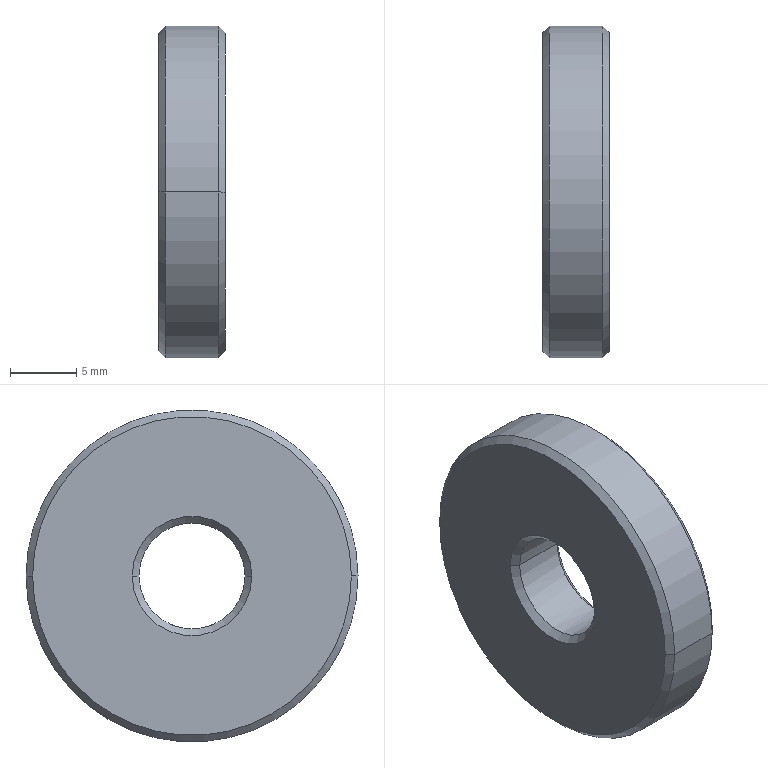Part | SolidWorks | features BaseBody 1 | 1 solid | 14 faces | box 5 x 25 x 25 mm | volume 2177 mm3 | cone 8 | cylinder 4 | plane 2 | commonest cylinder face diameters 8 x2 25 x2
STEP:
#1=CARTESIAN_POINT('',(5.,12.,0.));
#2=VERTEX_POINT('',#1);
#3=CARTESIAN_POINT('',(5.,-12.,0.));
#4=VERTEX_POINT('',#3);
#5=CARTESIAN_POINT('',(5.,0.,0.));
#6=DIRECTION('',(1.,0.,0.));
#7=DIRECTION('',(0.,-1.,0.));
#8=AXIS2_PLACEMENT_3D('',#5,#6,#7);
#9=CIRCLE('',#8,12.);
#10=EDGE_CURVE('',#2,#4,#9,.T.);
#11=ORIENTED_EDGE('',*,*,#10,.F.);
#12=CARTESIAN_POINT('',(4.5,12.5,0.));
#13=VERTEX_POINT('',#12);
#14=CARTESIAN_POINT('',(4.5,12.5,0.));
#15=DIRECTION('',(-0.7071,0.7071,0.));
#16=VECTOR('',#15,1000.);
#17=LINE('',#14,#16);
#18=EDGE_CURVE('',#2,#13,#17,.T.);
#19=ORIENTED_EDGE('',*,*,#18,.T.);
#20=CARTESIAN_POINT('',(4.5,-12.5,0.));
#21=VERTEX_POINT('',#20);
#22=CARTESIAN_POINT('',(4.5,0.,0.));
#23=DIRECTION('',(1.,0.,0.));
#24=DIRECTION('',(0.,-1.,0.));
#25=AXIS2_PLACEMENT_3D('',#22,#23,#24);
#26=CIRCLE('',#25,12.5);
#27=EDGE_CURVE('',#13,#21,#26,.T.);
#28=ORIENTED_EDGE('',*,*,#27,.T.);
#29=CARTESIAN_POINT('',(4.5,-12.5,0.));
#30=DIRECTION('',(-0.7071,-0.7071,0.));
#31=VECTOR('',#30,1000.);
#32=LINE('',#29,#31);
#33=EDGE_CURVE('',#4,#21,#32,.T.);
#34=ORIENTED_EDGE('',*,*,#33,.F.);
#35=EDGE_LOOP('',(#11,#19,#28,#34));
#36=FACE_OUTER_BOUND('',#35,.T.);
#37=CARTESIAN_POINT('',(4.5,0.,0.));
#38=DIRECTION('',(-1.,0.,0.));
#39=DIRECTION('',(0.,-1.,0.));
#40=AXIS2_PLACEMENT_3D('',#37,#38,#39);
#41=CONICAL_SURFACE('',#40,12.5,0.7854);
#42=ADVANCED_FACE('',(#36),#41,.T.);
#43=CARTESIAN_POINT('',(4.5,0.,4.));
#44=VERTEX_POINT('',#43);
#45=CARTESIAN_POINT('',(4.5,-4.,0.));
#46=VERTEX_POINT('',#45);
#47=CARTESIAN_POINT('',(4.5,0.,0.));
#48=DIRECTION('',(1.,0.,0.));
#49=DIRECTION('',(0.,1.,0.));
#50=AXIS2_PLACEMENT_3D('',#47,#48,#49);
#51=CIRCLE('',#50,4.);
#52=EDGE_CURVE('',#44,#46,#51,.T.);
#53=ORIENTED_EDGE('',*,*,#52,.F.);
#54=CARTESIAN_POINT('',(5.,0.,4.5));
#55=VERTEX_POINT('',#54);
#56=CARTESIAN_POINT('',(5.,0.,4.5));
#57=DIRECTION('',(0.7071,0.,0.7071));
#58=VECTOR('',#57,1000.);
#59=LINE('',#56,#58);
#60=EDGE_CURVE('',#44,#55,#59,.T.);
#61=ORIENTED_EDGE('',*,*,#60,.T.);
#62=CARTESIAN_POINT('',(5.,0.,-4.5));
#63=VERTEX_POINT('',#62);
#64=CARTESIAN_POINT('',(5.,0.,0.));
#65=DIRECTION('',(-1.,0.,0.));
#66=DIRECTION('',(0.,0.,-1.));
#67=AXIS2_PLACEMENT_3D('',#64,#65,#66);
#68=CIRCLE('',#67,4.5);
#69=EDGE_CURVE('',#63,#55,#68,.T.);
#70=ORIENTED_EDGE('',*,*,#69,.F.);
#71=CARTESIAN_POINT('',(4.5,0.,-4.));
#72=VERTEX_POINT('',#71);
#73=CARTESIAN_POINT('',(5.,0.,-4.5));
#74=DIRECTION('',(0.7071,0.,-0.7071));
#75=VECTOR('',#74,1000.);
#76=LINE('',#73,#75);
#77=EDGE_CURVE('',#72,#63,#76,.T.);
#78=ORIENTED_EDGE('',*,*,#77,.F.);
#79=CARTESIAN_POINT('',(4.5,0.,0.));
#80=DIRECTION('',(1.,0.,0.));
#81=DIRECTION('',(0.,1.,0.));
#82=AXIS2_PLACEMENT_3D('',#79,#80,#81);
#83=CIRCLE('',#82,4.);
#84=EDGE_CURVE('',#46,#72,#83,.T.);
#85=ORIENTED_EDGE('',*,*,#84,.F.);
#86=EDGE_LOOP('',(#53,#61,#70,#78,#85));
#87=FACE_OUTER_BOUND('',#86,.T.);
#88=CARTESIAN_POINT('',(5.,0.,0.));
#89=DIRECTION('',(1.,0.,0.));
#90=DIRECTION('',(0.,0.,-1.));
#91=AXIS2_PLACEMENT_3D('',#88,#89,#90);
#92=CONICAL_SURFACE('',#91,4.5,0.7854);
#93=ADVANCED_FACE('',(#87),#92,.F.);
#94=CARTESIAN_POINT('',(0.5,12.5,0.));
#95=VERTEX_POINT('',#94);
#96=CARTESIAN_POINT('',(0.5,-12.5,0.));
#97=VERTEX_POINT('',#96);
#98=CARTESIAN_POINT('',(0.5,0.,0.));
#99=DIRECTION('',(1.,0.,0.));
#100=DIRECTION('',(0.,1.,0.));
#101=AXIS2_PLACEMENT_3D('',#98,#99,#100);
#102=CIRCLE('',#101,12.5);
#103=EDGE_CURVE('',#95,#97,#102,.T.);
#104=ORIENTED_EDGE('',*,*,#103,.T.);
#105=CARTESIAN_POINT('',(-3.,-12.5,0.));
#106=DIRECTION('',(1.,0.,0.));
#107=VECTOR('',#106,1000.);
#108=LINE('',#105,#107);
#109=EDGE_CURVE('',#97,#21,#108,.T.);
#110=ORIENTED_EDGE('',*,*,#109,.T.);
#111=ORIENTED_EDGE('',*,*,#27,.F.);
#112=CARTESIAN_POINT('',(-3.,12.5,0.));
#113=DIRECTION('',(1.,0.,0.));
#114=VECTOR('',#113,1000.);
#115=LINE('',#112,#114);
#116=EDGE_CURVE('',#95,#13,#115,.T.);
#117=ORIENTED_EDGE('',*,*,#116,.F.);
#118=EDGE_LOOP('',(#104,#110,#111,#117));
#119=FACE_OUTER_BOUND('',#118,.T.);
#120=CARTESIAN_POINT('',(-3.,0.,0.));
#121=DIRECTION('',(1.,0.,0.));
#122=DIRECTION('',(0.,1.,0.));
#123=AXIS2_PLACEMENT_3D('',#120,#121,#122);
#124=CYLINDRICAL_SURFACE('',#123,12.5);
#125=ADVANCED_FACE('',(#119),#124,.T.);
#126=CARTESIAN_POINT('',(0.5,-4.,0.));
#127=VERTEX_POINT('',#126);
#128=CARTESIAN_POINT('',(0.5,4.,0.));
#129=VERTEX_POINT('',#128);
#130=CARTESIAN_POINT('',(0.5,0.,0.));
#131=DIRECTION('',(1.,0.,0.));
#132=DIRECTION('',(0.,1.,0.));
#133=AXIS2_PLACEMENT_3D('',#130,#131,#132);
#134=CIRCLE('',#133,4.);
#135=EDGE_CURVE('',#127,#129,#134,.T.);
#136=ORIENTED_EDGE('',*,*,#135,.F.);
#137=CARTESIAN_POINT('',(-3.,-4.,0.));
#138=DIRECTION('',(1.,0.,0.));
#139=VECTOR('',#138,1000.);
#140=LINE('',#137,#139);
#141=EDGE_CURVE('',#127,#46,#140,.T.);
#142=ORIENTED_EDGE('',*,*,#141,.T.);
#143=ORIENTED_EDGE('',*,*,#84,.T.);
#144=CARTESIAN_POINT('',(4.5,4.,0.));
#145=VERTEX_POINT('',#144);
#146=CARTESIAN_POINT('',(4.5,0.,0.));
#147=DIRECTION('',(1.,0.,0.));
#148=DIRECTION('',(0.,1.,0.));
#149=AXIS2_PLACEMENT_3D('',#146,#147,#148);
#150=CIRCLE('',#149,4.);
#151=EDGE_CURVE('',#72,#145,#150,.T.);
#152=ORIENTED_EDGE('',*,*,#151,.T.);
#153=CARTESIAN_POINT('',(-3.,4.,0.));
#154=DIRECTION('',(1.,0.,0.));
#155=VECTOR('',#154,1000.);
#156=LINE('',#153,#155);
#157=EDGE_CURVE('',#129,#145,#156,.T.);
#158=ORIENTED_EDGE('',*,*,#157,.F.);
#159=EDGE_LOOP('',(#136,#142,#143,#152,#158));
#160=FACE_OUTER_BOUND('',#159,.T.);
#161=CARTESIAN_POINT('',(-3.,0.,0.));
#162=DIRECTION('',(1.,0.,0.));
#163=DIRECTION('',(0.,1.,0.));
#164=AXIS2_PLACEMENT_3D('',#161,#162,#163);
#165=CYLINDRICAL_SURFACE('',#164,4.);
#166=ADVANCED_FACE('',(#160),#165,.F.);
#167=CARTESIAN_POINT('',(0.,12.,0.));
#168=VERTEX_POINT('',#167);
#169=CARTESIAN_POINT('',(0.,-12.,0.));
#170=VERTEX_POINT('',#169);
#171=CARTESIAN_POINT('',(0.,0.,0.));
#172=DIRECTION('',(1.,0.,0.));
#173=DIRECTION('',(0.,1.,0.));
#174=AXIS2_PLACEMENT_3D('',#171,#172,#173);
#175=CIRCLE('',#174,12.);
#176=EDGE_CURVE('',#168,#170,#175,.T.);
#177=ORIENTED_EDGE('',*,*,#176,.T.);
#178=CARTESIAN_POINT('',(0.5,-12.5,0.));
#179=DIRECTION('',(0.7071,-0.7071,0.));
#180=VECTOR('',#179,1000.);
#181=LINE('',#178,#180);
#182=EDGE_CURVE('',#170,#97,#181,.T.);
#183=ORIENTED_EDGE('',*,*,#182,.T.);
#184=ORIENTED_EDGE('',*,*,#103,.F.);
#185=CARTESIAN_POINT('',(0.5,12.5,0.));
#186=DIRECTION('',(0.7071,0.7071,0.));
#187=VECTOR('',#186,1000.);
#188=LINE('',#185,#187);
#189=EDGE_CURVE('',#168,#95,#188,.T.);
#190=ORIENTED_EDGE('',*,*,#189,.F.);
#191=EDGE_LOOP('',(#177,#183,#184,#190));
#192=FACE_OUTER_BOUND('',#191,.T.);
#193=CARTESIAN_POINT('',(0.5,0.,0.));
#194=DIRECTION('',(1.,0.,0.));
#195=DIRECTION('',(0.,1.,0.));
#196=AXIS2_PLACEMENT_3D('',#193,#194,#195);
#197=CONICAL_SURFACE('',#196,12.5,0.7854);
#198=ADVANCED_FACE('',(#192),#197,.T.);
#199=ORIENTED_EDGE('',*,*,#135,.T.);
#200=CARTESIAN_POINT('',(0.,4.5,0.));
#201=VERTEX_POINT('',#200);
#202=CARTESIAN_POINT('',(0.,4.5,0.));
#203=DIRECTION('',(-0.7071,0.7071,0.));
#204=VECTOR('',#203,1000.);
#205=LINE('',#202,#204);
#206=EDGE_CURVE('',#129,#201,#205,.T.);
#207=ORIENTED_EDGE('',*,*,#206,.T.);
#208=CARTESIAN_POINT('',(0.,-4.5,0.));
#209=VERTEX_POINT('',#208);
#210=CARTESIAN_POINT('',(0.,0.,0.));
#211=DIRECTION('',(1.,0.,0.));
#212=DIRECTION('',(0.,-1.,0.));
#213=AXIS2_PLACEMENT_3D('',#210,#211,#212);
#214=CIRCLE('',#213,4.5);
#215=EDGE_CURVE('',#209,#201,#214,.T.);
#216=ORIENTED_EDGE('',*,*,#215,.F.);
#217=CARTESIAN_POINT('',(0.,-4.5,0.));
#218=DIRECTION('',(-0.7071,-0.7071,0.));
#219=VECTOR('',#218,1000.);
#220=LINE('',#217,#219);
#221=EDGE_CURVE('',#127,#209,#220,.T.);
#222=ORIENTED_EDGE('',*,*,#221,.F.);
#223=EDGE_LOOP('',(#199,#207,#216,#222));
#224=FACE_OUTER_BOUND('',#223,.T.);
#225=CARTESIAN_POINT('',(0.,0.,0.));
#226=DIRECTION('',(-1.,0.,0.));
#227=DIRECTION('',(0.,-1.,0.));
#228=AXIS2_PLACEMENT_3D('',#225,#226,#227);
#229=CONICAL_SURFACE('',#228,4.5,0.7854);
#230=ADVANCED_FACE('',(#224),#229,.F.);
#231=CARTESIAN_POINT('',(5.,0.,0.));
#232=DIRECTION('',(1.,0.,0.));
#233=DIRECTION('',(0.,-1.,0.));
#234=AXIS2_PLACEMENT_3D('',#231,#232,#233);
#235=CIRCLE('',#234,12.);
#236=EDGE_CURVE('',#4,#2,#235,.T.);
#237=ORIENTED_EDGE('',*,*,#236,.T.);
#238=ORIENTED_EDGE('',*,*,#10,.T.);
#239=EDGE_LOOP('',(#237,#238));
#240=FACE_OUTER_BOUND('',#239,.T.);
#241=ORIENTED_EDGE('',*,*,#69,.T.);
#242=CARTESIAN_POINT('',(5.,0.,0.));
#243=DIRECTION('',(-1.,0.,0.));
#244=DIRECTION('',(0.,0.,-1.));
#245=AXIS2_PLACEMENT_3D('',#242,#243,#244);
#246=CIRCLE('',#245,4.5);
#247=EDGE_CURVE('',#55,#63,#246,.T.);
#248=ORIENTED_EDGE('',*,*,#247,.T.);
#249=EDGE_LOOP('',(#241,#248));
#250=FACE_BOUND('',#249,.T.);
#251=CARTESIAN_POINT('',(5.,-12.,0.));
#252=DIRECTION('',(1.,0.,0.));
#253=DIRECTION('',(0.,1.,0.));
#254=AXIS2_PLACEMENT_3D('',#251,#252,#253);
#255=PLANE('',#254);
#256=ADVANCED_FACE('',(#240,#250),#255,.T.);
#257=ORIENTED_EDGE('',*,*,#18,.F.);
#258=ORIENTED_EDGE('',*,*,#236,.F.);
#259=ORIENTED_EDGE('',*,*,#33,.T.);
#260=CARTESIAN_POINT('',(4.5,0.,0.));
#261=DIRECTION('',(1.,0.,0.));
#262=DIRECTION('',(0.,-1.,0.));
#263=AXIS2_PLACEMENT_3D('',#260,#261,#262);
#264=CIRCLE('',#263,12.5);
#265=EDGE_CURVE('',#21,#13,#264,.T.);
#266=ORIENTED_EDGE('',*,*,#265,.T.);
#267=EDGE_LOOP('',(#257,#258,#259,#266));
#268=FACE_OUTER_BOUND('',#267,.T.);
#269=CARTESIAN_POINT('',(4.5,0.,0.));
#270=DIRECTION('',(-1.,0.,0.));
#271=DIRECTION('',(0.,-1.,0.));
#272=AXIS2_PLACEMENT_3D('',#269,#270,#271);
#273=CONICAL_SURFACE('',#272,12.5,0.7854);
#274=ADVANCED_FACE('',(#268),#273,.T.);
#275=ORIENTED_EDGE('',*,*,#60,.F.);
#276=CARTESIAN_POINT('',(4.5,0.,0.));
#277=DIRECTION('',(1.,0.,0.));
#278=DIRECTION('',(0.,1.,0.));
#279=AXIS2_PLACEMENT_3D('',#276,#277,#278);
#280=CIRCLE('',#279,4.);
#281=EDGE_CURVE('',#145,#44,#280,.T.);
#282=ORIENTED_EDGE('',*,*,#281,.F.);
#283=ORIENTED_EDGE('',*,*,#151,.F.);
#284=ORIENTED_EDGE('',*,*,#77,.T.);
#285=ORIENTED_EDGE('',*,*,#247,.F.);
#286=EDGE_LOOP('',(#275,#282,#283,#284,#285));
#287=FACE_OUTER_BOUND('',#286,.T.);
#288=CARTESIAN_POINT('',(5.,0.,0.));
#289=DIRECTION('',(1.,0.,0.));
#290=DIRECTION('',(0.,0.,-1.));
#291=AXIS2_PLACEMENT_3D('',#288,#289,#290);
#292=CONICAL_SURFACE('',#291,4.5,0.7854);
#293=ADVANCED_FACE('',(#287),#292,.F.);
#294=ORIENTED_EDGE('',*,*,#109,.F.);
#295=CARTESIAN_POINT('',(0.5,0.,0.));
#296=DIRECTION('',(1.,0.,0.));
#297=DIRECTION('',(0.,1.,0.));
#298=AXIS2_PLACEMENT_3D('',#295,#296,#297);
#299=CIRCLE('',#298,12.5);
#300=EDGE_CURVE('',#97,#95,#299,.T.);
#301=ORIENTED_EDGE('',*,*,#300,.T.);
#302=ORIENTED_EDGE('',*,*,#116,.T.);
#303=ORIENTED_EDGE('',*,*,#265,.F.);
#304=EDGE_LOOP('',(#294,#301,#302,#303));
#305=FACE_OUTER_BOUND('',#304,.T.);
#306=CARTESIAN_POINT('',(-3.,0.,0.));
#307=DIRECTION('',(1.,0.,0.));
#308=DIRECTION('',(0.,1.,0.));
#309=AXIS2_PLACEMENT_3D('',#306,#307,#308);
#310=CYLINDRICAL_SURFACE('',#309,12.5);
#311=ADVANCED_FACE('',(#305),#310,.T.);
#312=ORIENTED_EDGE('',*,*,#141,.F.);
#313=CARTESIAN_POINT('',(0.5,0.,0.));
#314=DIRECTION('',(1.,0.,0.));
#315=DIRECTION('',(0.,1.,0.));
#316=AXIS2_PLACEMENT_3D('',#313,#314,#315);
#317=CIRCLE('',#316,4.);
#318=EDGE_CURVE('',#129,#127,#317,.T.);
#319=ORIENTED_EDGE('',*,*,#318,.F.);
#320=ORIENTED_EDGE('',*,*,#157,.T.);
#321=ORIENTED_EDGE('',*,*,#281,.T.);
#322=ORIENTED_EDGE('',*,*,#52,.T.);
#323=EDGE_LOOP('',(#312,#319,#320,#321,#322));
#324=FACE_OUTER_BOUND('',#323,.T.);
#325=CARTESIAN_POINT('',(-3.,0.,0.));
#326=DIRECTION('',(1.,0.,0.));
#327=DIRECTION('',(0.,1.,0.));
#328=AXIS2_PLACEMENT_3D('',#325,#326,#327);
#329=CYLINDRICAL_SURFACE('',#328,4.);
#330=ADVANCED_FACE('',(#324),#329,.F.);
#331=ORIENTED_EDGE('',*,*,#182,.F.);
#332=CARTESIAN_POINT('',(0.,0.,0.));
#333=DIRECTION('',(1.,0.,0.));
#334=DIRECTION('',(0.,1.,0.));
#335=AXIS2_PLACEMENT_3D('',#332,#333,#334);
#336=CIRCLE('',#335,12.);
#337=EDGE_CURVE('',#170,#168,#336,.T.);
#338=ORIENTED_EDGE('',*,*,#337,.T.);
#339=ORIENTED_EDGE('',*,*,#189,.T.);
#340=ORIENTED_EDGE('',*,*,#300,.F.);
#341=EDGE_LOOP('',(#331,#338,#339,#340));
#342=FACE_OUTER_BOUND('',#341,.T.);
#343=CARTESIAN_POINT('',(0.5,0.,0.));
#344=DIRECTION('',(1.,0.,0.));
#345=DIRECTION('',(0.,1.,0.));
#346=AXIS2_PLACEMENT_3D('',#343,#344,#345);
#347=CONICAL_SURFACE('',#346,12.5,0.7854);
#348=ADVANCED_FACE('',(#342),#347,.T.);
#349=ORIENTED_EDGE('',*,*,#206,.F.);
#350=ORIENTED_EDGE('',*,*,#318,.T.);
#351=ORIENTED_EDGE('',*,*,#221,.T.);
#352=CARTESIAN_POINT('',(0.,0.,0.));
#353=DIRECTION('',(1.,0.,0.));
#354=DIRECTION('',(0.,-1.,0.));
#355=AXIS2_PLACEMENT_3D('',#352,#353,#354);
#356=CIRCLE('',#355,4.5);
#357=EDGE_CURVE('',#201,#209,#356,.T.);
#358=ORIENTED_EDGE('',*,*,#357,.F.);
#359=EDGE_LOOP('',(#349,#350,#351,#358));
#360=FACE_OUTER_BOUND('',#359,.T.);
#361=CARTESIAN_POINT('',(0.,0.,0.));
#362=DIRECTION('',(-1.,0.,0.));
#363=DIRECTION('',(0.,-1.,0.));
#364=AXIS2_PLACEMENT_3D('',#361,#362,#363);
#365=CONICAL_SURFACE('',#364,4.5,0.7854);
#366=ADVANCED_FACE('',(#360),#365,.F.);
#367=ORIENTED_EDGE('',*,*,#215,.T.);
#368=ORIENTED_EDGE('',*,*,#357,.T.);
#369=EDGE_LOOP('',(#367,#368));
#370=FACE_BOUND('',#369,.T.);
#371=ORIENTED_EDGE('',*,*,#176,.F.);
#372=ORIENTED_EDGE('',*,*,#337,.F.);
#373=EDGE_LOOP('',(#371,#372));
#374=FACE_OUTER_BOUND('',#373,.T.);
#375=CARTESIAN_POINT('',(0.,-4.5,0.));
#376=DIRECTION('',(-1.,0.,0.));
#377=DIRECTION('',(0.,-1.,0.));
#378=AXIS2_PLACEMENT_3D('',#375,#376,#377);
#379=PLANE('',#378);
#380=ADVANCED_FACE('',(#370,#374),#379,.T.);
#381=CLOSED_SHELL('',(#42,#93,#125,#166,#198,#230,#256,#274,#293,#311,#330,#348,#366,#380));
#382=MANIFOLD_SOLID_BREP('',#381);
#383=CARTESIAN_POINT('',(0.,0.,0.));
#384=DIRECTION('',(0.,0.,1.));
#385=DIRECTION('',(1.,0.,0.));
#386=AXIS2_PLACEMENT_3D('',#383,#384,#385);
#387=(LENGTH_UNIT()NAMED_UNIT(*)SI_UNIT(.MILLI.,.METRE.));
#388=UNCERTAINTY_MEASURE_WITH_UNIT(LENGTH_MEASURE(0.00001),#387,'','');
#389=(NAMED_UNIT(*)PLANE_ANGLE_UNIT()SI_UNIT($,.RADIAN.));
#390=(NAMED_UNIT(*)SI_UNIT($,.STERADIAN.)SOLID_ANGLE_UNIT());
#391=(GEOMETRIC_REPRESENTATION_CONTEXT(3)GLOBAL_UNCERTAINTY_ASSIGNED_CONTEXT((#388))GLOBAL_UNIT_ASSIGNED_CONTEXT((#387,#389,#390))REPRESENTATION_CONTEXT('',''));
#392=ADVANCED_BREP_SHAPE_REPRESENTATION('',(#382,#386),#391);